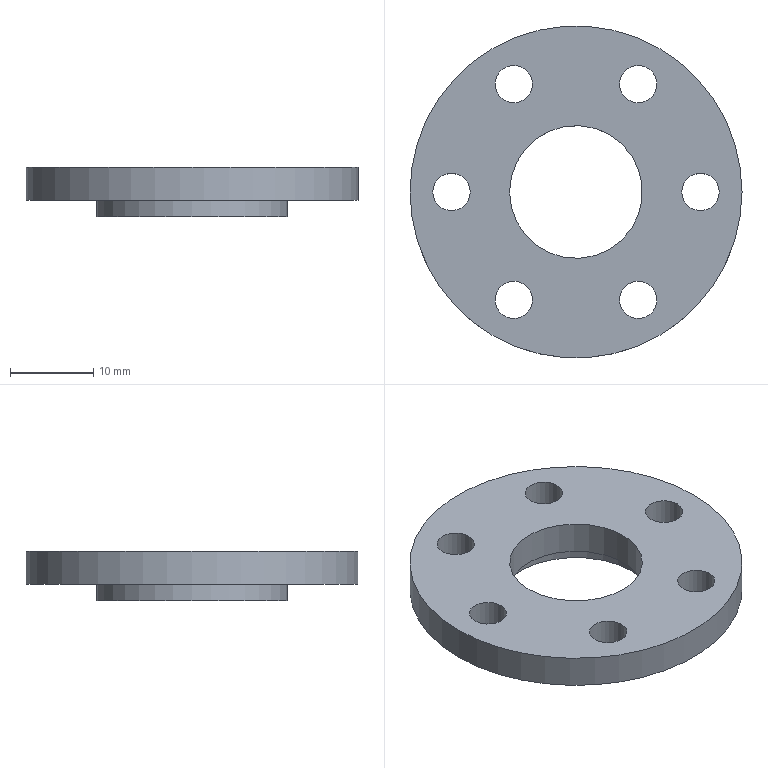Part | STEP file | zhouchenyagai1 | 1 solid | 14 faces | box 40 x 40 x 6 mm | volume 4104 mm3 | cylinder 10 | plane 4 | commonest cylinder face diameters 4.5 x6 16 x1 19 x1 23 x1 40 x1
STEP:
#1=CARTESIAN_POINT('',(0.,0.,0.));
#2=DIRECTION('',(0.,0.,1.));
#3=DIRECTION('',(1.,0.,0.));
#4=AXIS2_PLACEMENT_3D('',#1,#2,#3);
#5=CARTESIAN_POINT('',(-9.75,12.99,4.));
#6=VERTEX_POINT('',#5);
#7=CARTESIAN_POINT('',(-7.5,12.99,4.));
#8=DIRECTION('',(0.,0.,-1.));
#9=DIRECTION('',(-1.,0.,0.));
#10=AXIS2_PLACEMENT_3D('',#7,#8,#9);
#11=CIRCLE('',#10,2.25);
#12=CARTESIAN_POINT('',(0.,0.,4.));
#13=DIRECTION('',(0.,0.,1.));
#14=DIRECTION('',(1.,0.,0.));
#15=AXIS2_PLACEMENT_3D('',#12,#13,#14);
#16=PLANE('',#15);
#17=CARTESIAN_POINT('',(-9.75,12.99));
#18=CARTESIAN_POINT('',(-9.75,16.887));
#19=CARTESIAN_POINT('',(-6.375,14.939));
#20=CARTESIAN_POINT('',(-3.,12.99));
#21=CARTESIAN_POINT('',(-6.375,11.042));
#22=CARTESIAN_POINT('',(-9.75,9.093));
#23=CARTESIAN_POINT('',(-9.75,12.99));
#24=(BOUNDED_CURVE()B_SPLINE_CURVE(2,(#17,#18,#19,#20,#21,#22,#23),.UNSPECIFIED.,.T.,.F.)B_SPLINE_CURVE_WITH_KNOTS((1,2,2,2,2,1),(-2.094,0.,2.094,4.189,6.283,8.378),.UNSPECIFIED.)CURVE()GEOMETRIC_REPRESENTATION_ITEM()RATIONAL_B_SPLINE_CURVE((1.,0.5,1.,0.5,1.,0.5,1.))REPRESENTATION_ITEM(''));
#25=(GEOMETRIC_REPRESENTATION_CONTEXT(2)PARAMETRIC_REPRESENTATION_CONTEXT()REPRESENTATION_CONTEXT('',''));
#26=DEFINITIONAL_REPRESENTATION('',(#24),#25);
#27=PCURVE('',#16,#26);
#28=CARTESIAN_POINT('',(-7.5,12.99,4.));
#29=DIRECTION('',(0.,0.,-1.));
#30=DIRECTION('',(-1.,0.,0.));
#31=AXIS2_PLACEMENT_3D('',#28,#29,#30);
#32=CYLINDRICAL_SURFACE('',#31,2.25);
#33=CARTESIAN_POINT('',(0.,0.));
#34=DIRECTION('',(1.,0.));
#35=VECTOR('',#34,1.);
#36=LINE('',#33,#35);
#37=(GEOMETRIC_REPRESENTATION_CONTEXT(2)PARAMETRIC_REPRESENTATION_CONTEXT()REPRESENTATION_CONTEXT('',''));
#38=DEFINITIONAL_REPRESENTATION('',(#36),#37);
#39=PCURVE('',#32,#38);
#40=SURFACE_CURVE('',#11,(#27,#39),.PCURVE_S1.);
#41=EDGE_CURVE('',#6,#6,#40,.T.);
#42=ORIENTED_EDGE('',*,*,#41,.T.);
#43=EDGE_LOOP('',(#42));
#44=FACE_BOUND('',#43,.T.);
#45=CARTESIAN_POINT('',(12.75,0.,4.));
#46=VERTEX_POINT('',#45);
#47=CARTESIAN_POINT('',(15.,0.,4.));
#48=DIRECTION('',(0.,0.,-1.));
#49=DIRECTION('',(-1.,0.,0.));
#50=AXIS2_PLACEMENT_3D('',#47,#48,#49);
#51=CIRCLE('',#50,2.25);
#52=CARTESIAN_POINT('',(12.75,0.));
#53=CARTESIAN_POINT('',(12.75,3.897));
#54=CARTESIAN_POINT('',(16.125,1.949));
#55=CARTESIAN_POINT('',(19.5,0.));
#56=CARTESIAN_POINT('',(16.125,-1.949));
#57=CARTESIAN_POINT('',(12.75,-3.897));
#58=CARTESIAN_POINT('',(12.75,0.));
#59=(BOUNDED_CURVE()B_SPLINE_CURVE(2,(#52,#53,#54,#55,#56,#57,#58),.UNSPECIFIED.,.T.,.F.)B_SPLINE_CURVE_WITH_KNOTS((1,2,2,2,2,1),(-2.094,0.,2.094,4.189,6.283,8.378),.UNSPECIFIED.)CURVE()GEOMETRIC_REPRESENTATION_ITEM()RATIONAL_B_SPLINE_CURVE((1.,0.5,1.,0.5,1.,0.5,1.))REPRESENTATION_ITEM(''));
#60=(GEOMETRIC_REPRESENTATION_CONTEXT(2)PARAMETRIC_REPRESENTATION_CONTEXT()REPRESENTATION_CONTEXT('',''));
#61=DEFINITIONAL_REPRESENTATION('',(#59),#60);
#62=PCURVE('',#16,#61);
#63=CARTESIAN_POINT('',(15.,0.,4.));
#64=DIRECTION('',(0.,0.,-1.));
#65=DIRECTION('',(-1.,0.,0.));
#66=AXIS2_PLACEMENT_3D('',#63,#64,#65);
#67=CYLINDRICAL_SURFACE('',#66,2.25);
#68=CARTESIAN_POINT('',(0.,0.));
#69=DIRECTION('',(1.,0.));
#70=VECTOR('',#69,1.);
#71=LINE('',#68,#70);
#72=(GEOMETRIC_REPRESENTATION_CONTEXT(2)PARAMETRIC_REPRESENTATION_CONTEXT()REPRESENTATION_CONTEXT('',''));
#73=DEFINITIONAL_REPRESENTATION('',(#71),#72);
#74=PCURVE('',#67,#73);
#75=SURFACE_CURVE('',#51,(#62,#74),.PCURVE_S1.);
#76=EDGE_CURVE('',#46,#46,#75,.T.);
#77=ORIENTED_EDGE('',*,*,#76,.T.);
#78=EDGE_LOOP('',(#77));
#79=FACE_BOUND('',#78,.T.);
#80=CARTESIAN_POINT('',(-9.75,-12.99,4.));
#81=VERTEX_POINT('',#80);
#82=CARTESIAN_POINT('',(-7.5,-12.99,4.));
#83=DIRECTION('',(0.,0.,-1.));
#84=DIRECTION('',(-1.,0.,0.));
#85=AXIS2_PLACEMENT_3D('',#82,#83,#84);
#86=CIRCLE('',#85,2.25);
#87=CARTESIAN_POINT('',(-9.75,-12.99));
#88=CARTESIAN_POINT('',(-9.75,-9.093));
#89=CARTESIAN_POINT('',(-6.375,-11.042));
#90=CARTESIAN_POINT('',(-3.,-12.99));
#91=CARTESIAN_POINT('',(-6.375,-14.939));
#92=CARTESIAN_POINT('',(-9.75,-16.887));
#93=CARTESIAN_POINT('',(-9.75,-12.99));
#94=(BOUNDED_CURVE()B_SPLINE_CURVE(2,(#87,#88,#89,#90,#91,#92,#93),.UNSPECIFIED.,.T.,.F.)B_SPLINE_CURVE_WITH_KNOTS((1,2,2,2,2,1),(-2.094,0.,2.094,4.189,6.283,8.378),.UNSPECIFIED.)CURVE()GEOMETRIC_REPRESENTATION_ITEM()RATIONAL_B_SPLINE_CURVE((1.,0.5,1.,0.5,1.,0.5,1.))REPRESENTATION_ITEM(''));
#95=(GEOMETRIC_REPRESENTATION_CONTEXT(2)PARAMETRIC_REPRESENTATION_CONTEXT()REPRESENTATION_CONTEXT('',''));
#96=DEFINITIONAL_REPRESENTATION('',(#94),#95);
#97=PCURVE('',#16,#96);
#98=CARTESIAN_POINT('',(-7.5,-12.99,4.));
#99=DIRECTION('',(0.,0.,-1.));
#100=DIRECTION('',(-1.,0.,0.));
#101=AXIS2_PLACEMENT_3D('',#98,#99,#100);
#102=CYLINDRICAL_SURFACE('',#101,2.25);
#103=CARTESIAN_POINT('',(0.,0.));
#104=DIRECTION('',(1.,0.));
#105=VECTOR('',#104,1.);
#106=LINE('',#103,#105);
#107=(GEOMETRIC_REPRESENTATION_CONTEXT(2)PARAMETRIC_REPRESENTATION_CONTEXT()REPRESENTATION_CONTEXT('',''));
#108=DEFINITIONAL_REPRESENTATION('',(#106),#107);
#109=PCURVE('',#102,#108);
#110=SURFACE_CURVE('',#86,(#97,#109),.PCURVE_S1.);
#111=EDGE_CURVE('',#81,#81,#110,.T.);
#112=ORIENTED_EDGE('',*,*,#111,.T.);
#113=EDGE_LOOP('',(#112));
#114=FACE_BOUND('',#113,.T.);
#115=CARTESIAN_POINT('',(-8.,0.,4.));
#116=VERTEX_POINT('',#115);
#117=CARTESIAN_POINT('',(0.,0.,4.));
#118=DIRECTION('',(0.,0.,-1.));
#119=DIRECTION('',(-1.,0.,0.));
#120=AXIS2_PLACEMENT_3D('',#117,#118,#119);
#121=CIRCLE('',#120,8.);
#122=CARTESIAN_POINT('',(-8.,0.));
#123=CARTESIAN_POINT('',(-8.,13.856));
#124=CARTESIAN_POINT('',(4.,6.928));
#125=CARTESIAN_POINT('',(16.,0.));
#126=CARTESIAN_POINT('',(4.,-6.928));
#127=CARTESIAN_POINT('',(-8.,-13.856));
#128=CARTESIAN_POINT('',(-8.,0.));
#129=(BOUNDED_CURVE()B_SPLINE_CURVE(2,(#122,#123,#124,#125,#126,#127,#128),.UNSPECIFIED.,.T.,.F.)B_SPLINE_CURVE_WITH_KNOTS((1,2,2,2,2,1),(-2.094,0.,2.094,4.189,6.283,8.378),.UNSPECIFIED.)CURVE()GEOMETRIC_REPRESENTATION_ITEM()RATIONAL_B_SPLINE_CURVE((1.,0.5,1.,0.5,1.,0.5,1.))REPRESENTATION_ITEM(''));
#130=(GEOMETRIC_REPRESENTATION_CONTEXT(2)PARAMETRIC_REPRESENTATION_CONTEXT()REPRESENTATION_CONTEXT('',''));
#131=DEFINITIONAL_REPRESENTATION('',(#129),#130);
#132=PCURVE('',#16,#131);
#133=CARTESIAN_POINT('',(0.,0.,4.));
#134=DIRECTION('',(0.,0.,-1.));
#135=DIRECTION('',(-1.,0.,0.));
#136=AXIS2_PLACEMENT_3D('',#133,#134,#135);
#137=CYLINDRICAL_SURFACE('',#136,8.);
#138=CARTESIAN_POINT('',(0.,0.));
#139=DIRECTION('',(1.,0.));
#140=VECTOR('',#139,1.);
#141=LINE('',#138,#140);
#142=(GEOMETRIC_REPRESENTATION_CONTEXT(2)PARAMETRIC_REPRESENTATION_CONTEXT()REPRESENTATION_CONTEXT('',''));
#143=DEFINITIONAL_REPRESENTATION('',(#141),#142);
#144=PCURVE('',#137,#143);
#145=SURFACE_CURVE('',#121,(#132,#144),.PCURVE_S1.);
#146=EDGE_CURVE('',#116,#116,#145,.T.);
#147=ORIENTED_EDGE('',*,*,#146,.T.);
#148=EDGE_LOOP('',(#147));
#149=FACE_BOUND('',#148,.T.);
#150=CARTESIAN_POINT('',(-20.,0.,4.));
#151=VERTEX_POINT('',#150);
#152=CARTESIAN_POINT('',(0.,0.,4.));
#153=DIRECTION('',(0.,0.,1.));
#154=DIRECTION('',(-1.,0.,0.));
#155=AXIS2_PLACEMENT_3D('',#152,#153,#154);
#156=CIRCLE('',#155,20.);
#157=CARTESIAN_POINT('',(0.,0.));
#158=DIRECTION('',(-1.,0.));
#159=AXIS2_PLACEMENT_2D('',#157,#158);
#160=CIRCLE('',#159,20.);
#161=(GEOMETRIC_REPRESENTATION_CONTEXT(2)PARAMETRIC_REPRESENTATION_CONTEXT()REPRESENTATION_CONTEXT('',''));
#162=DEFINITIONAL_REPRESENTATION('',(#160),#161);
#163=PCURVE('',#16,#162);
#164=CARTESIAN_POINT('',(0.,0.,4.));
#165=DIRECTION('',(0.,0.,-1.));
#166=DIRECTION('',(-1.,0.,0.));
#167=AXIS2_PLACEMENT_3D('',#164,#165,#166);
#168=CYLINDRICAL_SURFACE('',#167,20.);
#169=CARTESIAN_POINT('',(6.283,0.));
#170=DIRECTION('',(-1.,0.));
#171=VECTOR('',#170,1.);
#172=LINE('',#169,#171);
#173=(GEOMETRIC_REPRESENTATION_CONTEXT(2)PARAMETRIC_REPRESENTATION_CONTEXT()REPRESENTATION_CONTEXT('',''));
#174=DEFINITIONAL_REPRESENTATION('',(#172),#173);
#175=PCURVE('',#168,#174);
#176=SURFACE_CURVE('',#156,(#163,#175),.PCURVE_S1.);
#177=EDGE_CURVE('',#151,#151,#176,.T.);
#178=ORIENTED_EDGE('',*,*,#177,.T.);
#179=EDGE_LOOP('',(#178));
#180=FACE_BOUND('',#179,.T.);
#181=CARTESIAN_POINT('',(-17.25,0.,4.));
#182=VERTEX_POINT('',#181);
#183=CARTESIAN_POINT('',(-15.,0.,4.));
#184=DIRECTION('',(0.,0.,-1.));
#185=DIRECTION('',(-1.,0.,0.));
#186=AXIS2_PLACEMENT_3D('',#183,#184,#185);
#187=CIRCLE('',#186,2.25);
#188=CARTESIAN_POINT('',(-17.25,0.));
#189=CARTESIAN_POINT('',(-17.25,3.897));
#190=CARTESIAN_POINT('',(-13.875,1.949));
#191=CARTESIAN_POINT('',(-10.5,0.));
#192=CARTESIAN_POINT('',(-13.875,-1.949));
#193=CARTESIAN_POINT('',(-17.25,-3.897));
#194=CARTESIAN_POINT('',(-17.25,0.));
#195=(BOUNDED_CURVE()B_SPLINE_CURVE(2,(#188,#189,#190,#191,#192,#193,#194),.UNSPECIFIED.,.T.,.F.)B_SPLINE_CURVE_WITH_KNOTS((1,2,2,2,2,1),(-2.094,0.,2.094,4.189,6.283,8.378),.UNSPECIFIED.)CURVE()GEOMETRIC_REPRESENTATION_ITEM()RATIONAL_B_SPLINE_CURVE((1.,0.5,1.,0.5,1.,0.5,1.))REPRESENTATION_ITEM(''));
#196=(GEOMETRIC_REPRESENTATION_CONTEXT(2)PARAMETRIC_REPRESENTATION_CONTEXT()REPRESENTATION_CONTEXT('',''));
#197=DEFINITIONAL_REPRESENTATION('',(#195),#196);
#198=PCURVE('',#16,#197);
#199=CARTESIAN_POINT('',(-15.,0.,4.));
#200=DIRECTION('',(0.,0.,-1.));
#201=DIRECTION('',(-1.,0.,0.));
#202=AXIS2_PLACEMENT_3D('',#199,#200,#201);
#203=CYLINDRICAL_SURFACE('',#202,2.25);
#204=CARTESIAN_POINT('',(0.,0.));
#205=DIRECTION('',(1.,0.));
#206=VECTOR('',#205,1.);
#207=LINE('',#204,#206);
#208=(GEOMETRIC_REPRESENTATION_CONTEXT(2)PARAMETRIC_REPRESENTATION_CONTEXT()REPRESENTATION_CONTEXT('',''));
#209=DEFINITIONAL_REPRESENTATION('',(#207),#208);
#210=PCURVE('',#203,#209);
#211=SURFACE_CURVE('',#187,(#198,#210),.PCURVE_S1.);
#212=EDGE_CURVE('',#182,#182,#211,.T.);
#213=ORIENTED_EDGE('',*,*,#212,.T.);
#214=EDGE_LOOP('',(#213));
#215=FACE_BOUND('',#214,.T.);
#216=CARTESIAN_POINT('',(5.25,-12.99,4.));
#217=VERTEX_POINT('',#216);
#218=CARTESIAN_POINT('',(7.5,-12.99,4.));
#219=DIRECTION('',(0.,0.,-1.));
#220=DIRECTION('',(-1.,0.,0.));
#221=AXIS2_PLACEMENT_3D('',#218,#219,#220);
#222=CIRCLE('',#221,2.25);
#223=CARTESIAN_POINT('',(5.25,-12.99));
#224=CARTESIAN_POINT('',(5.25,-9.093));
#225=CARTESIAN_POINT('',(8.625,-11.042));
#226=CARTESIAN_POINT('',(12.,-12.99));
#227=CARTESIAN_POINT('',(8.625,-14.939));
#228=CARTESIAN_POINT('',(5.25,-16.887));
#229=CARTESIAN_POINT('',(5.25,-12.99));
#230=(BOUNDED_CURVE()B_SPLINE_CURVE(2,(#223,#224,#225,#226,#227,#228,#229),.UNSPECIFIED.,.T.,.F.)B_SPLINE_CURVE_WITH_KNOTS((1,2,2,2,2,1),(-2.094,0.,2.094,4.189,6.283,8.378),.UNSPECIFIED.)CURVE()GEOMETRIC_REPRESENTATION_ITEM()RATIONAL_B_SPLINE_CURVE((1.,0.5,1.,0.5,1.,0.5,1.))REPRESENTATION_ITEM(''));
#231=(GEOMETRIC_REPRESENTATION_CONTEXT(2)PARAMETRIC_REPRESENTATION_CONTEXT()REPRESENTATION_CONTEXT('',''));
#232=DEFINITIONAL_REPRESENTATION('',(#230),#231);
#233=PCURVE('',#16,#232);
#234=CARTESIAN_POINT('',(7.5,-12.99,4.));
#235=DIRECTION('',(0.,0.,-1.));
#236=DIRECTION('',(-1.,0.,0.));
#237=AXIS2_PLACEMENT_3D('',#234,#235,#236);
#238=CYLINDRICAL_SURFACE('',#237,2.25);
#239=CARTESIAN_POINT('',(0.,0.));
#240=DIRECTION('',(1.,0.));
#241=VECTOR('',#240,1.);
#242=LINE('',#239,#241);
#243=(GEOMETRIC_REPRESENTATION_CONTEXT(2)PARAMETRIC_REPRESENTATION_CONTEXT()REPRESENTATION_CONTEXT('',''));
#244=DEFINITIONAL_REPRESENTATION('',(#242),#243);
#245=PCURVE('',#238,#244);
#246=SURFACE_CURVE('',#222,(#233,#245),.PCURVE_S1.);
#247=EDGE_CURVE('',#217,#217,#246,.T.);
#248=ORIENTED_EDGE('',*,*,#247,.T.);
#249=EDGE_LOOP('',(#248));
#250=FACE_BOUND('',#249,.T.);
#251=CARTESIAN_POINT('',(5.25,12.99,4.));
#252=VERTEX_POINT('',#251);
#253=CARTESIAN_POINT('',(7.5,12.99,4.));
#254=DIRECTION('',(0.,0.,-1.));
#255=DIRECTION('',(-1.,0.,0.));
#256=AXIS2_PLACEMENT_3D('',#253,#254,#255);
#257=CIRCLE('',#256,2.25);
#258=CARTESIAN_POINT('',(5.25,12.99));
#259=CARTESIAN_POINT('',(5.25,16.887));
#260=CARTESIAN_POINT('',(8.625,14.939));
#261=CARTESIAN_POINT('',(12.,12.99));
#262=CARTESIAN_POINT('',(8.625,11.042));
#263=CARTESIAN_POINT('',(5.25,9.093));
#264=CARTESIAN_POINT('',(5.25,12.99));
#265=(BOUNDED_CURVE()B_SPLINE_CURVE(2,(#258,#259,#260,#261,#262,#263,#264),.UNSPECIFIED.,.T.,.F.)B_SPLINE_CURVE_WITH_KNOTS((1,2,2,2,2,1),(-2.094,0.,2.094,4.189,6.283,8.378),.UNSPECIFIED.)CURVE()GEOMETRIC_REPRESENTATION_ITEM()RATIONAL_B_SPLINE_CURVE((1.,0.5,1.,0.5,1.,0.5,1.))REPRESENTATION_ITEM(''));
#266=(GEOMETRIC_REPRESENTATION_CONTEXT(2)PARAMETRIC_REPRESENTATION_CONTEXT()REPRESENTATION_CONTEXT('',''));
#267=DEFINITIONAL_REPRESENTATION('',(#265),#266);
#268=PCURVE('',#16,#267);
#269=CARTESIAN_POINT('',(7.5,12.99,4.));
#270=DIRECTION('',(0.,0.,-1.));
#271=DIRECTION('',(-1.,0.,0.));
#272=AXIS2_PLACEMENT_3D('',#269,#270,#271);
#273=CYLINDRICAL_SURFACE('',#272,2.25);
#274=CARTESIAN_POINT('',(0.,0.));
#275=DIRECTION('',(1.,0.));
#276=VECTOR('',#275,1.);
#277=LINE('',#274,#276);
#278=(GEOMETRIC_REPRESENTATION_CONTEXT(2)PARAMETRIC_REPRESENTATION_CONTEXT()REPRESENTATION_CONTEXT('',''));
#279=DEFINITIONAL_REPRESENTATION('',(#277),#278);
#280=PCURVE('',#273,#279);
#281=SURFACE_CURVE('',#257,(#268,#280),.PCURVE_S1.);
#282=EDGE_CURVE('',#252,#252,#281,.T.);
#283=ORIENTED_EDGE('',*,*,#282,.T.);
#284=EDGE_LOOP('',(#283));
#285=FACE_BOUND('',#284,.T.);
#286=ADVANCED_FACE('',(#44,#79,#114,#149,#180,#215,#250,#285),#16,.T.);
#287=ORIENTED_EDGE('',*,*,#41,.T.);
#288=CARTESIAN_POINT('',(-9.75,12.99,0.));
#289=VERTEX_POINT('',#288);
#290=CARTESIAN_POINT('',(-9.75,12.99,4.));
#291=CARTESIAN_POINT('',(-9.75,12.99,0.));
#292=B_SPLINE_CURVE_WITH_KNOTS('',1,(#290,#291),.UNSPECIFIED.,.F.,.F.,(2,2),(0.,4.),.PIECEWISE_BEZIER_KNOTS.);
#293=CARTESIAN_POINT('',(6.283,0.));
#294=DIRECTION('',(0.,1.));
#295=VECTOR('',#294,1.);
#296=LINE('',#293,#295);
#297=(GEOMETRIC_REPRESENTATION_CONTEXT(2)PARAMETRIC_REPRESENTATION_CONTEXT()REPRESENTATION_CONTEXT('',''));
#298=DEFINITIONAL_REPRESENTATION('',(#296),#297);
#299=PCURVE('',#32,#298);
#300=CARTESIAN_POINT('',(0.,0.));
#301=DIRECTION('',(0.,1.));
#302=VECTOR('',#301,1.);
#303=LINE('',#300,#302);
#304=(GEOMETRIC_REPRESENTATION_CONTEXT(2)PARAMETRIC_REPRESENTATION_CONTEXT()REPRESENTATION_CONTEXT('',''));
#305=DEFINITIONAL_REPRESENTATION('',(#303),#304);
#306=PCURVE('',#32,#305);
#307=SEAM_CURVE('',#292,(#299,#306),.PCURVE_S1.);
#308=EDGE_CURVE('',#6,#289,#307,.T.);
#309=ORIENTED_EDGE('',*,*,#308,.T.);
#310=CARTESIAN_POINT('',(-7.5,12.99,0.));
#311=DIRECTION('',(0.,0.,1.));
#312=DIRECTION('',(-1.,0.,0.));
#313=AXIS2_PLACEMENT_3D('',#310,#311,#312);
#314=CIRCLE('',#313,2.25);
#315=CARTESIAN_POINT('',(6.283,4.));
#316=DIRECTION('',(-1.,0.));
#317=VECTOR('',#316,1.);
#318=LINE('',#315,#317);
#319=(GEOMETRIC_REPRESENTATION_CONTEXT(2)PARAMETRIC_REPRESENTATION_CONTEXT()REPRESENTATION_CONTEXT('',''));
#320=DEFINITIONAL_REPRESENTATION('',(#318),#319);
#321=PCURVE('',#32,#320);
#322=CARTESIAN_POINT('',(0.,0.,0.));
#323=DIRECTION('',(0.,0.,1.));
#324=DIRECTION('',(1.,0.,0.));
#325=AXIS2_PLACEMENT_3D('',#322,#323,#324);
#326=PLANE('',#325);
#327=CARTESIAN_POINT('',(-7.5,12.99));
#328=DIRECTION('',(-1.,0.));
#329=AXIS2_PLACEMENT_2D('',#327,#328);
#330=CIRCLE('',#329,2.25);
#331=(GEOMETRIC_REPRESENTATION_CONTEXT(2)PARAMETRIC_REPRESENTATION_CONTEXT()REPRESENTATION_CONTEXT('',''));
#332=DEFINITIONAL_REPRESENTATION('',(#330),#331);
#333=PCURVE('',#326,#332);
#334=SURFACE_CURVE('',#314,(#321,#333),.PCURVE_S1.);
#335=EDGE_CURVE('',#289,#289,#334,.T.);
#336=ORIENTED_EDGE('',*,*,#335,.T.);
#337=ORIENTED_EDGE('',*,*,#308,.F.);
#338=EDGE_LOOP('',(#287,#309,#336,#337));
#339=FACE_BOUND('',#338,.F.);
#340=ADVANCED_FACE('',(#339),#32,.F.);
#341=ORIENTED_EDGE('',*,*,#76,.T.);
#342=CARTESIAN_POINT('',(12.75,0.,0.));
#343=VERTEX_POINT('',#342);
#344=CARTESIAN_POINT('',(12.75,0.,4.));
#345=CARTESIAN_POINT('',(12.75,0.,0.));
#346=B_SPLINE_CURVE_WITH_KNOTS('',1,(#344,#345),.UNSPECIFIED.,.F.,.F.,(2,2),(0.,4.),.PIECEWISE_BEZIER_KNOTS.);
#347=CARTESIAN_POINT('',(6.283,0.));
#348=DIRECTION('',(0.,1.));
#349=VECTOR('',#348,1.);
#350=LINE('',#347,#349);
#351=(GEOMETRIC_REPRESENTATION_CONTEXT(2)PARAMETRIC_REPRESENTATION_CONTEXT()REPRESENTATION_CONTEXT('',''));
#352=DEFINITIONAL_REPRESENTATION('',(#350),#351);
#353=PCURVE('',#67,#352);
#354=CARTESIAN_POINT('',(0.,0.));
#355=DIRECTION('',(0.,1.));
#356=VECTOR('',#355,1.);
#357=LINE('',#354,#356);
#358=(GEOMETRIC_REPRESENTATION_CONTEXT(2)PARAMETRIC_REPRESENTATION_CONTEXT()REPRESENTATION_CONTEXT('',''));
#359=DEFINITIONAL_REPRESENTATION('',(#357),#358);
#360=PCURVE('',#67,#359);
#361=SEAM_CURVE('',#346,(#353,#360),.PCURVE_S1.);
#362=EDGE_CURVE('',#46,#343,#361,.T.);
#363=ORIENTED_EDGE('',*,*,#362,.T.);
#364=CARTESIAN_POINT('',(15.,0.,0.));
#365=DIRECTION('',(0.,0.,1.));
#366=DIRECTION('',(-1.,0.,0.));
#367=AXIS2_PLACEMENT_3D('',#364,#365,#366);
#368=CIRCLE('',#367,2.25);
#369=CARTESIAN_POINT('',(6.283,4.));
#370=DIRECTION('',(-1.,0.));
#371=VECTOR('',#370,1.);
#372=LINE('',#369,#371);
#373=(GEOMETRIC_REPRESENTATION_CONTEXT(2)PARAMETRIC_REPRESENTATION_CONTEXT()REPRESENTATION_CONTEXT('',''));
#374=DEFINITIONAL_REPRESENTATION('',(#372),#373);
#375=PCURVE('',#67,#374);
#376=CARTESIAN_POINT('',(15.,0.));
#377=DIRECTION('',(-1.,0.));
#378=AXIS2_PLACEMENT_2D('',#376,#377);
#379=CIRCLE('',#378,2.25);
#380=(GEOMETRIC_REPRESENTATION_CONTEXT(2)PARAMETRIC_REPRESENTATION_CONTEXT()REPRESENTATION_CONTEXT('',''));
#381=DEFINITIONAL_REPRESENTATION('',(#379),#380);
#382=PCURVE('',#326,#381);
#383=SURFACE_CURVE('',#368,(#375,#382),.PCURVE_S1.);
#384=EDGE_CURVE('',#343,#343,#383,.T.);
#385=ORIENTED_EDGE('',*,*,#384,.T.);
#386=ORIENTED_EDGE('',*,*,#362,.F.);
#387=EDGE_LOOP('',(#341,#363,#385,#386));
#388=FACE_BOUND('',#387,.F.);
#389=ADVANCED_FACE('',(#388),#67,.F.);
#390=ORIENTED_EDGE('',*,*,#111,.T.);
#391=CARTESIAN_POINT('',(-9.75,-12.99,0.));
#392=VERTEX_POINT('',#391);
#393=CARTESIAN_POINT('',(-9.75,-12.99,4.));
#394=CARTESIAN_POINT('',(-9.75,-12.99,0.));
#395=B_SPLINE_CURVE_WITH_KNOTS('',1,(#393,#394),.UNSPECIFIED.,.F.,.F.,(2,2),(0.,4.),.PIECEWISE_BEZIER_KNOTS.);
#396=CARTESIAN_POINT('',(6.283,0.));
#397=DIRECTION('',(0.,1.));
#398=VECTOR('',#397,1.);
#399=LINE('',#396,#398);
#400=(GEOMETRIC_REPRESENTATION_CONTEXT(2)PARAMETRIC_REPRESENTATION_CONTEXT()REPRESENTATION_CONTEXT('',''));
#401=DEFINITIONAL_REPRESENTATION('',(#399),#400);
#402=PCURVE('',#102,#401);
#403=CARTESIAN_POINT('',(0.,0.));
#404=DIRECTION('',(0.,1.));
#405=VECTOR('',#404,1.);
#406=LINE('',#403,#405);
#407=(GEOMETRIC_REPRESENTATION_CONTEXT(2)PARAMETRIC_REPRESENTATION_CONTEXT()REPRESENTATION_CONTEXT('',''));
#408=DEFINITIONAL_REPRESENTATION('',(#406),#407);
#409=PCURVE('',#102,#408);
#410=SEAM_CURVE('',#395,(#402,#409),.PCURVE_S1.);
#411=EDGE_CURVE('',#81,#392,#410,.T.);
#412=ORIENTED_EDGE('',*,*,#411,.T.);
#413=CARTESIAN_POINT('',(-7.5,-12.99,0.));
#414=DIRECTION('',(0.,0.,1.));
#415=DIRECTION('',(-1.,0.,0.));
#416=AXIS2_PLACEMENT_3D('',#413,#414,#415);
#417=CIRCLE('',#416,2.25);
#418=CARTESIAN_POINT('',(6.283,4.));
#419=DIRECTION('',(-1.,0.));
#420=VECTOR('',#419,1.);
#421=LINE('',#418,#420);
#422=(GEOMETRIC_REPRESENTATION_CONTEXT(2)PARAMETRIC_REPRESENTATION_CONTEXT()REPRESENTATION_CONTEXT('',''));
#423=DEFINITIONAL_REPRESENTATION('',(#421),#422);
#424=PCURVE('',#102,#423);
#425=CARTESIAN_POINT('',(-7.5,-12.99));
#426=DIRECTION('',(-1.,0.));
#427=AXIS2_PLACEMENT_2D('',#425,#426);
#428=CIRCLE('',#427,2.25);
#429=(GEOMETRIC_REPRESENTATION_CONTEXT(2)PARAMETRIC_REPRESENTATION_CONTEXT()REPRESENTATION_CONTEXT('',''));
#430=DEFINITIONAL_REPRESENTATION('',(#428),#429);
#431=PCURVE('',#326,#430);
#432=SURFACE_CURVE('',#417,(#424,#431),.PCURVE_S1.);
#433=EDGE_CURVE('',#392,#392,#432,.T.);
#434=ORIENTED_EDGE('',*,*,#433,.T.);
#435=ORIENTED_EDGE('',*,*,#411,.F.);
#436=EDGE_LOOP('',(#390,#412,#434,#435));
#437=FACE_BOUND('',#436,.F.);
#438=ADVANCED_FACE('',(#437),#102,.F.);
#439=ORIENTED_EDGE('',*,*,#146,.T.);
#440=CARTESIAN_POINT('',(-8.,0.,0.));
#441=VERTEX_POINT('',#440);
#442=CARTESIAN_POINT('',(-8.,0.,4.));
#443=CARTESIAN_POINT('',(-8.,0.,0.));
#444=B_SPLINE_CURVE_WITH_KNOTS('',1,(#442,#443),.UNSPECIFIED.,.F.,.F.,(2,2),(0.,4.),.PIECEWISE_BEZIER_KNOTS.);
#445=CARTESIAN_POINT('',(6.283,0.));
#446=DIRECTION('',(0.,1.));
#447=VECTOR('',#446,1.);
#448=LINE('',#445,#447);
#449=(GEOMETRIC_REPRESENTATION_CONTEXT(2)PARAMETRIC_REPRESENTATION_CONTEXT()REPRESENTATION_CONTEXT('',''));
#450=DEFINITIONAL_REPRESENTATION('',(#448),#449);
#451=PCURVE('',#137,#450);
#452=CARTESIAN_POINT('',(0.,0.));
#453=DIRECTION('',(0.,1.));
#454=VECTOR('',#453,1.);
#455=LINE('',#452,#454);
#456=(GEOMETRIC_REPRESENTATION_CONTEXT(2)PARAMETRIC_REPRESENTATION_CONTEXT()REPRESENTATION_CONTEXT('',''));
#457=DEFINITIONAL_REPRESENTATION('',(#455),#456);
#458=PCURVE('',#137,#457);
#459=SEAM_CURVE('',#444,(#451,#458),.PCURVE_S1.);
#460=EDGE_CURVE('',#116,#441,#459,.T.);
#461=ORIENTED_EDGE('',*,*,#460,.T.);
#462=CARTESIAN_POINT('',(0.,0.,0.));
#463=DIRECTION('',(0.,0.,1.));
#464=DIRECTION('',(-1.,0.,0.));
#465=AXIS2_PLACEMENT_3D('',#462,#463,#464);
#466=CIRCLE('',#465,8.);
#467=CARTESIAN_POINT('',(6.283,4.));
#468=DIRECTION('',(-1.,0.));
#469=VECTOR('',#468,1.);
#470=LINE('',#467,#469);
#471=(GEOMETRIC_REPRESENTATION_CONTEXT(2)PARAMETRIC_REPRESENTATION_CONTEXT()REPRESENTATION_CONTEXT('',''));
#472=DEFINITIONAL_REPRESENTATION('',(#470),#471);
#473=PCURVE('',#137,#472);
#474=CARTESIAN_POINT('',(0.,0.,0.));
#475=DIRECTION('',(0.,0.,1.));
#476=DIRECTION('',(1.,0.,0.));
#477=AXIS2_PLACEMENT_3D('',#474,#475,#476);
#478=PLANE('',#477);
#479=CARTESIAN_POINT('',(0.,0.));
#480=DIRECTION('',(-1.,0.));
#481=AXIS2_PLACEMENT_2D('',#479,#480);
#482=CIRCLE('',#481,8.);
#483=(GEOMETRIC_REPRESENTATION_CONTEXT(2)PARAMETRIC_REPRESENTATION_CONTEXT()REPRESENTATION_CONTEXT('',''));
#484=DEFINITIONAL_REPRESENTATION('',(#482),#483);
#485=PCURVE('',#478,#484);
#486=SURFACE_CURVE('',#466,(#473,#485),.PCURVE_S1.);
#487=EDGE_CURVE('',#441,#441,#486,.T.);
#488=ORIENTED_EDGE('',*,*,#487,.T.);
#489=ORIENTED_EDGE('',*,*,#460,.F.);
#490=EDGE_LOOP('',(#439,#461,#488,#489));
#491=FACE_BOUND('',#490,.F.);
#492=ADVANCED_FACE('',(#491),#137,.F.);
#493=CARTESIAN_POINT('',(-20.,0.,0.));
#494=VERTEX_POINT('',#493);
#495=CARTESIAN_POINT('',(0.,0.,0.));
#496=DIRECTION('',(0.,0.,1.));
#497=DIRECTION('',(-1.,0.,0.));
#498=AXIS2_PLACEMENT_3D('',#495,#496,#497);
#499=CIRCLE('',#498,20.);
#500=CARTESIAN_POINT('',(6.283,4.));
#501=DIRECTION('',(-1.,0.));
#502=VECTOR('',#501,1.);
#503=LINE('',#500,#502);
#504=(GEOMETRIC_REPRESENTATION_CONTEXT(2)PARAMETRIC_REPRESENTATION_CONTEXT()REPRESENTATION_CONTEXT('',''));
#505=DEFINITIONAL_REPRESENTATION('',(#503),#504);
#506=PCURVE('',#168,#505);
#507=CARTESIAN_POINT('',(0.,0.));
#508=DIRECTION('',(-1.,0.));
#509=AXIS2_PLACEMENT_2D('',#507,#508);
#510=CIRCLE('',#509,20.);
#511=(GEOMETRIC_REPRESENTATION_CONTEXT(2)PARAMETRIC_REPRESENTATION_CONTEXT()REPRESENTATION_CONTEXT('',''));
#512=DEFINITIONAL_REPRESENTATION('',(#510),#511);
#513=PCURVE('',#326,#512);
#514=SURFACE_CURVE('',#499,(#506,#513),.PCURVE_S1.);
#515=EDGE_CURVE('',#494,#494,#514,.T.);
#516=ORIENTED_EDGE('',*,*,#515,.T.);
#517=CARTESIAN_POINT('',(-20.,0.,4.));
#518=CARTESIAN_POINT('',(-20.,0.,0.));
#519=B_SPLINE_CURVE_WITH_KNOTS('',1,(#517,#518),.UNSPECIFIED.,.F.,.F.,(2,2),(0.,4.),.PIECEWISE_BEZIER_KNOTS.);
#520=CARTESIAN_POINT('',(0.,0.));
#521=DIRECTION('',(0.,1.));
#522=VECTOR('',#521,1.);
#523=LINE('',#520,#522);
#524=(GEOMETRIC_REPRESENTATION_CONTEXT(2)PARAMETRIC_REPRESENTATION_CONTEXT()REPRESENTATION_CONTEXT('',''));
#525=DEFINITIONAL_REPRESENTATION('',(#523),#524);
#526=PCURVE('',#168,#525);
#527=CARTESIAN_POINT('',(6.283,0.));
#528=DIRECTION('',(0.,1.));
#529=VECTOR('',#528,1.);
#530=LINE('',#527,#529);
#531=(GEOMETRIC_REPRESENTATION_CONTEXT(2)PARAMETRIC_REPRESENTATION_CONTEXT()REPRESENTATION_CONTEXT('',''));
#532=DEFINITIONAL_REPRESENTATION('',(#530),#531);
#533=PCURVE('',#168,#532);
#534=SEAM_CURVE('',#519,(#526,#533),.PCURVE_S1.);
#535=EDGE_CURVE('',#151,#494,#534,.T.);
#536=ORIENTED_EDGE('',*,*,#535,.F.);
#537=ORIENTED_EDGE('',*,*,#177,.F.);
#538=ORIENTED_EDGE('',*,*,#535,.T.);
#539=EDGE_LOOP('',(#516,#536,#537,#538));
#540=FACE_BOUND('',#539,.T.);
#541=ADVANCED_FACE('',(#540),#168,.T.);
#542=ORIENTED_EDGE('',*,*,#212,.T.);
#543=CARTESIAN_POINT('',(-17.25,0.,0.));
#544=VERTEX_POINT('',#543);
#545=CARTESIAN_POINT('',(-17.25,0.,4.));
#546=CARTESIAN_POINT('',(-17.25,0.,0.));
#547=B_SPLINE_CURVE_WITH_KNOTS('',1,(#545,#546),.UNSPECIFIED.,.F.,.F.,(2,2),(0.,4.),.PIECEWISE_BEZIER_KNOTS.);
#548=CARTESIAN_POINT('',(6.283,0.));
#549=DIRECTION('',(0.,1.));
#550=VECTOR('',#549,1.);
#551=LINE('',#548,#550);
#552=(GEOMETRIC_REPRESENTATION_CONTEXT(2)PARAMETRIC_REPRESENTATION_CONTEXT()REPRESENTATION_CONTEXT('',''));
#553=DEFINITIONAL_REPRESENTATION('',(#551),#552);
#554=PCURVE('',#203,#553);
#555=CARTESIAN_POINT('',(0.,0.));
#556=DIRECTION('',(0.,1.));
#557=VECTOR('',#556,1.);
#558=LINE('',#555,#557);
#559=(GEOMETRIC_REPRESENTATION_CONTEXT(2)PARAMETRIC_REPRESENTATION_CONTEXT()REPRESENTATION_CONTEXT('',''));
#560=DEFINITIONAL_REPRESENTATION('',(#558),#559);
#561=PCURVE('',#203,#560);
#562=SEAM_CURVE('',#547,(#554,#561),.PCURVE_S1.);
#563=EDGE_CURVE('',#182,#544,#562,.T.);
#564=ORIENTED_EDGE('',*,*,#563,.T.);
#565=CARTESIAN_POINT('',(-15.,0.,0.));
#566=DIRECTION('',(0.,0.,1.));
#567=DIRECTION('',(-1.,0.,0.));
#568=AXIS2_PLACEMENT_3D('',#565,#566,#567);
#569=CIRCLE('',#568,2.25);
#570=CARTESIAN_POINT('',(6.283,4.));
#571=DIRECTION('',(-1.,0.));
#572=VECTOR('',#571,1.);
#573=LINE('',#570,#572);
#574=(GEOMETRIC_REPRESENTATION_CONTEXT(2)PARAMETRIC_REPRESENTATION_CONTEXT()REPRESENTATION_CONTEXT('',''));
#575=DEFINITIONAL_REPRESENTATION('',(#573),#574);
#576=PCURVE('',#203,#575);
#577=CARTESIAN_POINT('',(-15.,0.));
#578=DIRECTION('',(-1.,0.));
#579=AXIS2_PLACEMENT_2D('',#577,#578);
#580=CIRCLE('',#579,2.25);
#581=(GEOMETRIC_REPRESENTATION_CONTEXT(2)PARAMETRIC_REPRESENTATION_CONTEXT()REPRESENTATION_CONTEXT('',''));
#582=DEFINITIONAL_REPRESENTATION('',(#580),#581);
#583=PCURVE('',#326,#582);
#584=SURFACE_CURVE('',#569,(#576,#583),.PCURVE_S1.);
#585=EDGE_CURVE('',#544,#544,#584,.T.);
#586=ORIENTED_EDGE('',*,*,#585,.T.);
#587=ORIENTED_EDGE('',*,*,#563,.F.);
#588=EDGE_LOOP('',(#542,#564,#586,#587));
#589=FACE_BOUND('',#588,.F.);
#590=ADVANCED_FACE('',(#589),#203,.F.);
#591=ORIENTED_EDGE('',*,*,#247,.T.);
#592=CARTESIAN_POINT('',(5.25,-12.99,0.));
#593=VERTEX_POINT('',#592);
#594=CARTESIAN_POINT('',(5.25,-12.99,4.));
#595=CARTESIAN_POINT('',(5.25,-12.99,0.));
#596=B_SPLINE_CURVE_WITH_KNOTS('',1,(#594,#595),.UNSPECIFIED.,.F.,.F.,(2,2),(0.,4.),.PIECEWISE_BEZIER_KNOTS.);
#597=CARTESIAN_POINT('',(6.283,0.));
#598=DIRECTION('',(0.,1.));
#599=VECTOR('',#598,1.);
#600=LINE('',#597,#599);
#601=(GEOMETRIC_REPRESENTATION_CONTEXT(2)PARAMETRIC_REPRESENTATION_CONTEXT()REPRESENTATION_CONTEXT('',''));
#602=DEFINITIONAL_REPRESENTATION('',(#600),#601);
#603=PCURVE('',#238,#602);
#604=CARTESIAN_POINT('',(0.,0.));
#605=DIRECTION('',(0.,1.));
#606=VECTOR('',#605,1.);
#607=LINE('',#604,#606);
#608=(GEOMETRIC_REPRESENTATION_CONTEXT(2)PARAMETRIC_REPRESENTATION_CONTEXT()REPRESENTATION_CONTEXT('',''));
#609=DEFINITIONAL_REPRESENTATION('',(#607),#608);
#610=PCURVE('',#238,#609);
#611=SEAM_CURVE('',#596,(#603,#610),.PCURVE_S1.);
#612=EDGE_CURVE('',#217,#593,#611,.T.);
#613=ORIENTED_EDGE('',*,*,#612,.T.);
#614=CARTESIAN_POINT('',(7.5,-12.99,0.));
#615=DIRECTION('',(0.,0.,1.));
#616=DIRECTION('',(-1.,0.,0.));
#617=AXIS2_PLACEMENT_3D('',#614,#615,#616);
#618=CIRCLE('',#617,2.25);
#619=CARTESIAN_POINT('',(6.283,4.));
#620=DIRECTION('',(-1.,0.));
#621=VECTOR('',#620,1.);
#622=LINE('',#619,#621);
#623=(GEOMETRIC_REPRESENTATION_CONTEXT(2)PARAMETRIC_REPRESENTATION_CONTEXT()REPRESENTATION_CONTEXT('',''));
#624=DEFINITIONAL_REPRESENTATION('',(#622),#623);
#625=PCURVE('',#238,#624);
#626=CARTESIAN_POINT('',(7.5,-12.99));
#627=DIRECTION('',(-1.,0.));
#628=AXIS2_PLACEMENT_2D('',#626,#627);
#629=CIRCLE('',#628,2.25);
#630=(GEOMETRIC_REPRESENTATION_CONTEXT(2)PARAMETRIC_REPRESENTATION_CONTEXT()REPRESENTATION_CONTEXT('',''));
#631=DEFINITIONAL_REPRESENTATION('',(#629),#630);
#632=PCURVE('',#326,#631);
#633=SURFACE_CURVE('',#618,(#625,#632),.PCURVE_S1.);
#634=EDGE_CURVE('',#593,#593,#633,.T.);
#635=ORIENTED_EDGE('',*,*,#634,.T.);
#636=ORIENTED_EDGE('',*,*,#612,.F.);
#637=EDGE_LOOP('',(#591,#613,#635,#636));
#638=FACE_BOUND('',#637,.F.);
#639=ADVANCED_FACE('',(#638),#238,.F.);
#640=ORIENTED_EDGE('',*,*,#282,.T.);
#641=CARTESIAN_POINT('',(5.25,12.99,0.));
#642=VERTEX_POINT('',#641);
#643=CARTESIAN_POINT('',(5.25,12.99,4.));
#644=CARTESIAN_POINT('',(5.25,12.99,0.));
#645=B_SPLINE_CURVE_WITH_KNOTS('',1,(#643,#644),.UNSPECIFIED.,.F.,.F.,(2,2),(0.,4.),.PIECEWISE_BEZIER_KNOTS.);
#646=CARTESIAN_POINT('',(6.283,0.));
#647=DIRECTION('',(0.,1.));
#648=VECTOR('',#647,1.);
#649=LINE('',#646,#648);
#650=(GEOMETRIC_REPRESENTATION_CONTEXT(2)PARAMETRIC_REPRESENTATION_CONTEXT()REPRESENTATION_CONTEXT('',''));
#651=DEFINITIONAL_REPRESENTATION('',(#649),#650);
#652=PCURVE('',#273,#651);
#653=CARTESIAN_POINT('',(0.,0.));
#654=DIRECTION('',(0.,1.));
#655=VECTOR('',#654,1.);
#656=LINE('',#653,#655);
#657=(GEOMETRIC_REPRESENTATION_CONTEXT(2)PARAMETRIC_REPRESENTATION_CONTEXT()REPRESENTATION_CONTEXT('',''));
#658=DEFINITIONAL_REPRESENTATION('',(#656),#657);
#659=PCURVE('',#273,#658);
#660=SEAM_CURVE('',#645,(#652,#659),.PCURVE_S1.);
#661=EDGE_CURVE('',#252,#642,#660,.T.);
#662=ORIENTED_EDGE('',*,*,#661,.T.);
#663=CARTESIAN_POINT('',(7.5,12.99,0.));
#664=DIRECTION('',(0.,0.,1.));
#665=DIRECTION('',(-1.,0.,0.));
#666=AXIS2_PLACEMENT_3D('',#663,#664,#665);
#667=CIRCLE('',#666,2.25);
#668=CARTESIAN_POINT('',(6.283,4.));
#669=DIRECTION('',(-1.,0.));
#670=VECTOR('',#669,1.);
#671=LINE('',#668,#670);
#672=(GEOMETRIC_REPRESENTATION_CONTEXT(2)PARAMETRIC_REPRESENTATION_CONTEXT()REPRESENTATION_CONTEXT('',''));
#673=DEFINITIONAL_REPRESENTATION('',(#671),#672);
#674=PCURVE('',#273,#673);
#675=CARTESIAN_POINT('',(7.5,12.99));
#676=DIRECTION('',(-1.,0.));
#677=AXIS2_PLACEMENT_2D('',#675,#676);
#678=CIRCLE('',#677,2.25);
#679=(GEOMETRIC_REPRESENTATION_CONTEXT(2)PARAMETRIC_REPRESENTATION_CONTEXT()REPRESENTATION_CONTEXT('',''));
#680=DEFINITIONAL_REPRESENTATION('',(#678),#679);
#681=PCURVE('',#326,#680);
#682=SURFACE_CURVE('',#667,(#674,#681),.PCURVE_S1.);
#683=EDGE_CURVE('',#642,#642,#682,.T.);
#684=ORIENTED_EDGE('',*,*,#683,.T.);
#685=ORIENTED_EDGE('',*,*,#661,.F.);
#686=EDGE_LOOP('',(#640,#662,#684,#685));
#687=FACE_BOUND('',#686,.F.);
#688=ADVANCED_FACE('',(#687),#273,.F.);
#689=ORIENTED_EDGE('',*,*,#335,.T.);
#690=EDGE_LOOP('',(#689));
#691=FACE_BOUND('',#690,.T.);
#692=ORIENTED_EDGE('',*,*,#683,.T.);
#693=EDGE_LOOP('',(#692));
#694=FACE_BOUND('',#693,.T.);
#695=ORIENTED_EDGE('',*,*,#384,.T.);
#696=EDGE_LOOP('',(#695));
#697=FACE_BOUND('',#696,.T.);
#698=ORIENTED_EDGE('',*,*,#634,.T.);
#699=EDGE_LOOP('',(#698));
#700=FACE_BOUND('',#699,.T.);
#701=ORIENTED_EDGE('',*,*,#433,.T.);
#702=EDGE_LOOP('',(#701));
#703=FACE_BOUND('',#702,.T.);
#704=ORIENTED_EDGE('',*,*,#585,.T.);
#705=EDGE_LOOP('',(#704));
#706=FACE_BOUND('',#705,.T.);
#707=ORIENTED_EDGE('',*,*,#515,.F.);
#708=EDGE_LOOP('',(#707));
#709=FACE_BOUND('',#708,.T.);
#710=CARTESIAN_POINT('',(11.5,0.,0.));
#711=VERTEX_POINT('',#710);
#712=CARTESIAN_POINT('',(0.,0.,0.));
#713=DIRECTION('',(0.,0.,-1.));
#714=DIRECTION('',(1.,0.,0.));
#715=AXIS2_PLACEMENT_3D('',#712,#713,#714);
#716=CIRCLE('',#715,11.5);
#717=CARTESIAN_POINT('',(11.5,0.));
#718=CARTESIAN_POINT('',(11.5,-19.919));
#719=CARTESIAN_POINT('',(-5.75,-9.959));
#720=CARTESIAN_POINT('',(-23.,0.));
#721=CARTESIAN_POINT('',(-5.75,9.959));
#722=CARTESIAN_POINT('',(11.5,19.919));
#723=CARTESIAN_POINT('',(11.5,0.));
#724=(BOUNDED_CURVE()B_SPLINE_CURVE(2,(#717,#718,#719,#720,#721,#722,#723),.UNSPECIFIED.,.T.,.F.)B_SPLINE_CURVE_WITH_KNOTS((1,2,2,2,2,1),(-2.094,0.,2.094,4.189,6.283,8.378),.UNSPECIFIED.)CURVE()GEOMETRIC_REPRESENTATION_ITEM()RATIONAL_B_SPLINE_CURVE((1.,0.5,1.,0.5,1.,0.5,1.))REPRESENTATION_ITEM(''));
#725=(GEOMETRIC_REPRESENTATION_CONTEXT(2)PARAMETRIC_REPRESENTATION_CONTEXT()REPRESENTATION_CONTEXT('',''));
#726=DEFINITIONAL_REPRESENTATION('',(#724),#725);
#727=PCURVE('',#326,#726);
#728=CARTESIAN_POINT('',(0.,0.,-2.));
#729=DIRECTION('',(0.,0.,1.));
#730=DIRECTION('',(1.,0.,0.));
#731=AXIS2_PLACEMENT_3D('',#728,#729,#730);
#732=CYLINDRICAL_SURFACE('',#731,11.5);
#733=CARTESIAN_POINT('',(6.283,2.));
#734=DIRECTION('',(-1.,0.));
#735=VECTOR('',#734,1.);
#736=LINE('',#733,#735);
#737=(GEOMETRIC_REPRESENTATION_CONTEXT(2)PARAMETRIC_REPRESENTATION_CONTEXT()REPRESENTATION_CONTEXT('',''));
#738=DEFINITIONAL_REPRESENTATION('',(#736),#737);
#739=PCURVE('',#732,#738);
#740=SURFACE_CURVE('',#716,(#727,#739),.PCURVE_S1.);
#741=EDGE_CURVE('',#711,#711,#740,.T.);
#742=ORIENTED_EDGE('',*,*,#741,.F.);
#743=EDGE_LOOP('',(#742));
#744=FACE_BOUND('',#743,.T.);
#745=ADVANCED_FACE('',(#691,#694,#697,#700,#703,#706,#709,#744),#326,.F.);
#746=CARTESIAN_POINT('',(9.5,0.,0.));
#747=VERTEX_POINT('',#746);
#748=CARTESIAN_POINT('',(0.,0.,0.));
#749=DIRECTION('',(0.,0.,1.));
#750=DIRECTION('',(1.,0.,0.));
#751=AXIS2_PLACEMENT_3D('',#748,#749,#750);
#752=CIRCLE('',#751,9.5);
#753=CARTESIAN_POINT('',(0.,0.));
#754=DIRECTION('',(1.,0.));
#755=AXIS2_PLACEMENT_2D('',#753,#754);
#756=CIRCLE('',#755,9.5);
#757=(GEOMETRIC_REPRESENTATION_CONTEXT(2)PARAMETRIC_REPRESENTATION_CONTEXT()REPRESENTATION_CONTEXT('',''));
#758=DEFINITIONAL_REPRESENTATION('',(#756),#757);
#759=PCURVE('',#478,#758);
#760=CARTESIAN_POINT('',(0.,0.,-2.));
#761=DIRECTION('',(0.,0.,1.));
#762=DIRECTION('',(1.,0.,0.));
#763=AXIS2_PLACEMENT_3D('',#760,#761,#762);
#764=CYLINDRICAL_SURFACE('',#763,9.5);
#765=CARTESIAN_POINT('',(0.,2.));
#766=DIRECTION('',(1.,0.));
#767=VECTOR('',#766,1.);
#768=LINE('',#765,#767);
#769=(GEOMETRIC_REPRESENTATION_CONTEXT(2)PARAMETRIC_REPRESENTATION_CONTEXT()REPRESENTATION_CONTEXT('',''));
#770=DEFINITIONAL_REPRESENTATION('',(#768),#769);
#771=PCURVE('',#764,#770);
#772=SURFACE_CURVE('',#752,(#759,#771),.PCURVE_S1.);
#773=EDGE_CURVE('',#747,#747,#772,.T.);
#774=ORIENTED_EDGE('',*,*,#773,.F.);
#775=EDGE_LOOP('',(#774));
#776=FACE_BOUND('',#775,.T.);
#777=ORIENTED_EDGE('',*,*,#487,.T.);
#778=EDGE_LOOP('',(#777));
#779=FACE_BOUND('',#778,.T.);
#780=ADVANCED_FACE('',(#776,#779),#478,.F.);
#781=CARTESIAN_POINT('',(11.5,0.,-2.));
#782=VERTEX_POINT('',#781);
#783=CARTESIAN_POINT('',(0.,0.,-2.));
#784=DIRECTION('',(0.,0.,1.));
#785=DIRECTION('',(1.,0.,0.));
#786=AXIS2_PLACEMENT_3D('',#783,#784,#785);
#787=CIRCLE('',#786,11.5);
#788=CARTESIAN_POINT('',(0.,0.));
#789=DIRECTION('',(1.,0.));
#790=VECTOR('',#789,1.);
#791=LINE('',#788,#790);
#792=(GEOMETRIC_REPRESENTATION_CONTEXT(2)PARAMETRIC_REPRESENTATION_CONTEXT()REPRESENTATION_CONTEXT('',''));
#793=DEFINITIONAL_REPRESENTATION('',(#791),#792);
#794=PCURVE('',#732,#793);
#795=CARTESIAN_POINT('',(0.,0.,-2.));
#796=DIRECTION('',(0.,0.,-1.));
#797=DIRECTION('',(-1.,0.,0.));
#798=AXIS2_PLACEMENT_3D('',#795,#796,#797);
#799=PLANE('',#798);
#800=CARTESIAN_POINT('',(-11.5,0.));
#801=CARTESIAN_POINT('',(-11.5,19.919));
#802=CARTESIAN_POINT('',(5.75,9.959));
#803=CARTESIAN_POINT('',(23.,0.));
#804=CARTESIAN_POINT('',(5.75,-9.959));
#805=CARTESIAN_POINT('',(-11.5,-19.919));
#806=CARTESIAN_POINT('',(-11.5,0.));
#807=(BOUNDED_CURVE()B_SPLINE_CURVE(2,(#800,#801,#802,#803,#804,#805,#806),.UNSPECIFIED.,.T.,.F.)B_SPLINE_CURVE_WITH_KNOTS((1,2,2,2,2,1),(-2.094,0.,2.094,4.189,6.283,8.378),.UNSPECIFIED.)CURVE()GEOMETRIC_REPRESENTATION_ITEM()RATIONAL_B_SPLINE_CURVE((1.,0.5,1.,0.5,1.,0.5,1.))REPRESENTATION_ITEM(''));
#808=(GEOMETRIC_REPRESENTATION_CONTEXT(2)PARAMETRIC_REPRESENTATION_CONTEXT()REPRESENTATION_CONTEXT('',''));
#809=DEFINITIONAL_REPRESENTATION('',(#807),#808);
#810=PCURVE('',#799,#809);
#811=SURFACE_CURVE('',#787,(#794,#810),.PCURVE_S1.);
#812=EDGE_CURVE('',#782,#782,#811,.T.);
#813=ORIENTED_EDGE('',*,*,#812,.T.);
#814=CARTESIAN_POINT('',(11.5,0.,-2.));
#815=CARTESIAN_POINT('',(11.5,0.,0.));
#816=B_SPLINE_CURVE_WITH_KNOTS('',1,(#814,#815),.UNSPECIFIED.,.F.,.F.,(2,2),(0.,2.),.PIECEWISE_BEZIER_KNOTS.);
#817=CARTESIAN_POINT('',(6.283,0.));
#818=DIRECTION('',(0.,1.));
#819=VECTOR('',#818,1.);
#820=LINE('',#817,#819);
#821=(GEOMETRIC_REPRESENTATION_CONTEXT(2)PARAMETRIC_REPRESENTATION_CONTEXT()REPRESENTATION_CONTEXT('',''));
#822=DEFINITIONAL_REPRESENTATION('',(#820),#821);
#823=PCURVE('',#732,#822);
#824=CARTESIAN_POINT('',(0.,0.));
#825=DIRECTION('',(0.,1.));
#826=VECTOR('',#825,1.);
#827=LINE('',#824,#826);
#828=(GEOMETRIC_REPRESENTATION_CONTEXT(2)PARAMETRIC_REPRESENTATION_CONTEXT()REPRESENTATION_CONTEXT('',''));
#829=DEFINITIONAL_REPRESENTATION('',(#827),#828);
#830=PCURVE('',#732,#829);
#831=SEAM_CURVE('',#816,(#823,#830),.PCURVE_S1.);
#832=EDGE_CURVE('',#782,#711,#831,.T.);
#833=ORIENTED_EDGE('',*,*,#832,.T.);
#834=ORIENTED_EDGE('',*,*,#741,.T.);
#835=ORIENTED_EDGE('',*,*,#832,.F.);
#836=EDGE_LOOP('',(#813,#833,#834,#835));
#837=FACE_BOUND('',#836,.T.);
#838=ADVANCED_FACE('',(#837),#732,.T.);
#839=ORIENTED_EDGE('',*,*,#773,.F.);
#840=CARTESIAN_POINT('',(9.5,0.,-2.));
#841=VERTEX_POINT('',#840);
#842=CARTESIAN_POINT('',(9.5,0.,-2.));
#843=CARTESIAN_POINT('',(9.5,0.,0.));
#844=B_SPLINE_CURVE_WITH_KNOTS('',1,(#842,#843),.UNSPECIFIED.,.F.,.F.,(2,2),(0.,2.),.PIECEWISE_BEZIER_KNOTS.);
#845=CARTESIAN_POINT('',(0.,0.));
#846=DIRECTION('',(0.,1.));
#847=VECTOR('',#846,1.);
#848=LINE('',#845,#847);
#849=(GEOMETRIC_REPRESENTATION_CONTEXT(2)PARAMETRIC_REPRESENTATION_CONTEXT()REPRESENTATION_CONTEXT('',''));
#850=DEFINITIONAL_REPRESENTATION('',(#848),#849);
#851=PCURVE('',#764,#850);
#852=CARTESIAN_POINT('',(6.283,0.));
#853=DIRECTION('',(0.,1.));
#854=VECTOR('',#853,1.);
#855=LINE('',#852,#854);
#856=(GEOMETRIC_REPRESENTATION_CONTEXT(2)PARAMETRIC_REPRESENTATION_CONTEXT()REPRESENTATION_CONTEXT('',''));
#857=DEFINITIONAL_REPRESENTATION('',(#855),#856);
#858=PCURVE('',#764,#857);
#859=SEAM_CURVE('',#844,(#851,#858),.PCURVE_S1.);
#860=EDGE_CURVE('',#841,#747,#859,.T.);
#861=ORIENTED_EDGE('',*,*,#860,.F.);
#862=CARTESIAN_POINT('',(0.,0.,-2.));
#863=DIRECTION('',(0.,0.,1.));
#864=DIRECTION('',(1.,0.,0.));
#865=AXIS2_PLACEMENT_3D('',#862,#863,#864);
#866=CIRCLE('',#865,9.5);
#867=CARTESIAN_POINT('',(0.,0.));
#868=DIRECTION('',(1.,0.));
#869=VECTOR('',#868,1.);
#870=LINE('',#867,#869);
#871=(GEOMETRIC_REPRESENTATION_CONTEXT(2)PARAMETRIC_REPRESENTATION_CONTEXT()REPRESENTATION_CONTEXT('',''));
#872=DEFINITIONAL_REPRESENTATION('',(#870),#871);
#873=PCURVE('',#764,#872);
#874=CARTESIAN_POINT('',(-9.5,0.));
#875=CARTESIAN_POINT('',(-9.5,16.454));
#876=CARTESIAN_POINT('',(4.75,8.227));
#877=CARTESIAN_POINT('',(19.,0.));
#878=CARTESIAN_POINT('',(4.75,-8.227));
#879=CARTESIAN_POINT('',(-9.5,-16.454));
#880=CARTESIAN_POINT('',(-9.5,0.));
#881=(BOUNDED_CURVE()B_SPLINE_CURVE(2,(#874,#875,#876,#877,#878,#879,#880),.UNSPECIFIED.,.T.,.F.)B_SPLINE_CURVE_WITH_KNOTS((1,2,2,2,2,1),(-2.094,0.,2.094,4.189,6.283,8.378),.UNSPECIFIED.)CURVE()GEOMETRIC_REPRESENTATION_ITEM()RATIONAL_B_SPLINE_CURVE((1.,0.5,1.,0.5,1.,0.5,1.))REPRESENTATION_ITEM(''));
#882=(GEOMETRIC_REPRESENTATION_CONTEXT(2)PARAMETRIC_REPRESENTATION_CONTEXT()REPRESENTATION_CONTEXT('',''));
#883=DEFINITIONAL_REPRESENTATION('',(#881),#882);
#884=PCURVE('',#799,#883);
#885=SURFACE_CURVE('',#866,(#873,#884),.PCURVE_S1.);
#886=EDGE_CURVE('',#841,#841,#885,.T.);
#887=ORIENTED_EDGE('',*,*,#886,.T.);
#888=ORIENTED_EDGE('',*,*,#860,.T.);
#889=EDGE_LOOP('',(#839,#861,#887,#888));
#890=FACE_BOUND('',#889,.F.);
#891=ADVANCED_FACE('',(#890),#764,.F.);
#892=ORIENTED_EDGE('',*,*,#886,.T.);
#893=EDGE_LOOP('',(#892));
#894=FACE_BOUND('',#893,.T.);
#895=ORIENTED_EDGE('',*,*,#812,.F.);
#896=EDGE_LOOP('',(#895));
#897=FACE_BOUND('',#896,.T.);
#898=ADVANCED_FACE('',(#894,#897),#799,.T.);
#899=CLOSED_SHELL('',(#286,#340,#389,#438,#492,#541,#590,#639,#688,#745,#780,#838,#891,#898));
#900=MANIFOLD_SOLID_BREP('',#899);
#901=(LENGTH_UNIT()NAMED_UNIT(*)SI_UNIT(.MILLI.,.METRE.));
#902=UNCERTAINTY_MEASURE_WITH_UNIT(LENGTH_MEASURE(0.00001),#901,'','');
#903=(NAMED_UNIT(*)PLANE_ANGLE_UNIT()SI_UNIT($,.RADIAN.));
#904=(NAMED_UNIT(*)SI_UNIT($,.STERADIAN.)SOLID_ANGLE_UNIT());
#905=(GEOMETRIC_REPRESENTATION_CONTEXT(3)GLOBAL_UNCERTAINTY_ASSIGNED_CONTEXT((#902))GLOBAL_UNIT_ASSIGNED_CONTEXT((#901,#903,#904))REPRESENTATION_CONTEXT('',''));
#906=ADVANCED_BREP_SHAPE_REPRESENTATION('',(#4,#900),#905);